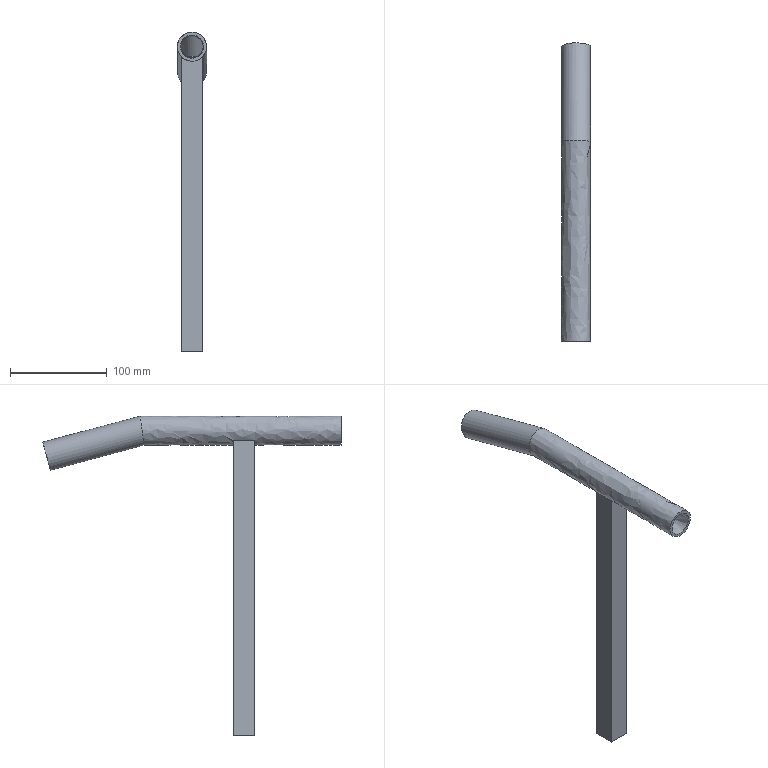Part | NX | features solid 2 | 1 solid | 22 faces | box 30 x 307.765 x 330 mm | volume 126218 mm3 | plane 15 | spline 7